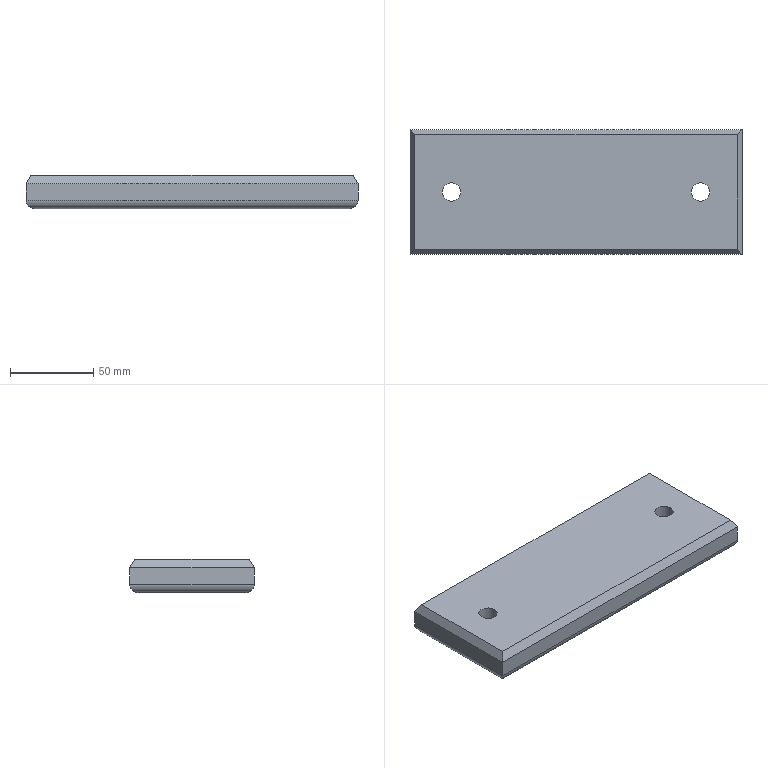Part | NX | features solid 2 | 1 solid | 22 faces | box 200 x 75 x 20 mm | volume 285510 mm3 | plane 12 | cylinder 8 | torus 2 | commonest cylinder face diameters 10 x4 11 x2 17.5 x2
STEP:
#1=CARTESIAN_POINT('',(110.,355.,205.));
#2=VERTEX_POINT('',#1);
#3=CARTESIAN_POINT('',(110.,355.,195.));
#4=VERTEX_POINT('',#3);
#5=CARTESIAN_POINT('',(110.,355.,210.));
#6=DIRECTION('',(0.,0.,-1.));
#7=VECTOR('',#6,1000.);
#8=LINE('',#5,#7);
#9=EDGE_CURVE('',#2,#4,#8,.T.);
#10=ORIENTED_EDGE('',*,*,#9,.F.);
#11=CARTESIAN_POINT('',(310.,355.,205.));
#12=VERTEX_POINT('',#11);
#13=CARTESIAN_POINT('',(230.,355.,205.));
#14=DIRECTION('',(1.,0.,0.));
#15=VECTOR('',#14,1000.);
#16=LINE('',#13,#15);
#17=EDGE_CURVE('',#2,#12,#16,.T.);
#18=ORIENTED_EDGE('',*,*,#17,.T.);
#19=CARTESIAN_POINT('',(310.,355.,195.));
#20=VERTEX_POINT('',#19);
#21=CARTESIAN_POINT('',(310.,355.,210.));
#22=DIRECTION('',(0.,0.,-1.));
#23=VECTOR('',#22,1000.);
#24=LINE('',#21,#23);
#25=EDGE_CURVE('',#12,#20,#24,.T.);
#26=ORIENTED_EDGE('',*,*,#25,.T.);
#27=CARTESIAN_POINT('',(110.,355.,195.));
#28=DIRECTION('',(-1.,0.,0.));
#29=VECTOR('',#28,1000.);
#30=LINE('',#27,#29);
#31=EDGE_CURVE('',#20,#4,#30,.T.);
#32=ORIENTED_EDGE('',*,*,#31,.T.);
#33=EDGE_LOOP('',(#10,#18,#26,#32));
#34=FACE_BOUND('',#33,.T.);
#35=CARTESIAN_POINT('',(230.,355.,210.));
#36=DIRECTION('',(0.,-1.,0.));
#37=DIRECTION('',(0.,0.,-1.));
#38=AXIS2_PLACEMENT_3D('',#35,#36,#37);
#39=PLANE('',#38);
#40=ADVANCED_FACE('',(#34),#39,.F.);
#41=CARTESIAN_POINT('',(110.,280.,205.));
#42=VERTEX_POINT('',#41);
#43=CARTESIAN_POINT('',(110.,280.,195.));
#44=VERTEX_POINT('',#43);
#45=CARTESIAN_POINT('',(110.,280.,210.));
#46=DIRECTION('',(0.,0.,-1.));
#47=VECTOR('',#46,1000.);
#48=LINE('',#45,#47);
#49=EDGE_CURVE('',#42,#44,#48,.T.);
#50=ORIENTED_EDGE('',*,*,#49,.F.);
#51=CARTESIAN_POINT('',(110.,355.,205.));
#52=DIRECTION('',(0.,1.,0.));
#53=VECTOR('',#52,1000.);
#54=LINE('',#51,#53);
#55=EDGE_CURVE('',#42,#2,#54,.T.);
#56=ORIENTED_EDGE('',*,*,#55,.T.);
#57=ORIENTED_EDGE('',*,*,#9,.T.);
#58=CARTESIAN_POINT('',(110.,280.,195.));
#59=DIRECTION('',(0.,-1.,0.));
#60=VECTOR('',#59,1000.);
#61=LINE('',#58,#60);
#62=EDGE_CURVE('',#4,#44,#61,.T.);
#63=ORIENTED_EDGE('',*,*,#62,.T.);
#64=EDGE_LOOP('',(#50,#56,#57,#63));
#65=FACE_BOUND('',#64,.T.);
#66=CARTESIAN_POINT('',(110.,355.,210.));
#67=DIRECTION('',(1.,0.,0.));
#68=DIRECTION('',(0.,0.,1.));
#69=AXIS2_PLACEMENT_3D('',#66,#67,#68);
#70=PLANE('',#69);
#71=ADVANCED_FACE('',(#65),#70,.F.);
#72=CARTESIAN_POINT('',(310.,280.,205.));
#73=VERTEX_POINT('',#72);
#74=CARTESIAN_POINT('',(310.,280.,195.));
#75=VERTEX_POINT('',#74);
#76=CARTESIAN_POINT('',(310.,280.,210.));
#77=DIRECTION('',(0.,0.,-1.));
#78=VECTOR('',#77,1000.);
#79=LINE('',#76,#78);
#80=EDGE_CURVE('',#73,#75,#79,.T.);
#81=ORIENTED_EDGE('',*,*,#80,.F.);
#82=CARTESIAN_POINT('',(110.,280.,205.));
#83=DIRECTION('',(-1.,0.,0.));
#84=VECTOR('',#83,1000.);
#85=LINE('',#82,#84);
#86=EDGE_CURVE('',#73,#42,#85,.T.);
#87=ORIENTED_EDGE('',*,*,#86,.T.);
#88=ORIENTED_EDGE('',*,*,#49,.T.);
#89=CARTESIAN_POINT('',(230.,280.,195.));
#90=DIRECTION('',(-1.,0.,0.));
#91=VECTOR('',#90,1000.);
#92=LINE('',#89,#91);
#93=EDGE_CURVE('',#44,#75,#92,.F.);
#94=ORIENTED_EDGE('',*,*,#93,.T.);
#95=EDGE_LOOP('',(#81,#87,#88,#94));
#96=FACE_BOUND('',#95,.T.);
#97=CARTESIAN_POINT('',(230.,280.,210.));
#98=DIRECTION('',(0.,-1.,0.));
#99=DIRECTION('',(0.,0.,-1.));
#100=AXIS2_PLACEMENT_3D('',#97,#98,#99);
#101=PLANE('',#100);
#102=ADVANCED_FACE('',(#96),#101,.T.);
#103=ORIENTED_EDGE('',*,*,#25,.F.);
#104=CARTESIAN_POINT('',(310.,280.,205.));
#105=DIRECTION('',(0.,-1.,0.));
#106=VECTOR('',#105,1000.);
#107=LINE('',#104,#106);
#108=EDGE_CURVE('',#12,#73,#107,.T.);
#109=ORIENTED_EDGE('',*,*,#108,.T.);
#110=ORIENTED_EDGE('',*,*,#80,.T.);
#111=CARTESIAN_POINT('',(310.,355.,195.));
#112=DIRECTION('',(0.,-1.,0.));
#113=VECTOR('',#112,1000.);
#114=LINE('',#111,#113);
#115=EDGE_CURVE('',#75,#20,#114,.F.);
#116=ORIENTED_EDGE('',*,*,#115,.T.);
#117=EDGE_LOOP('',(#103,#109,#110,#116));
#118=FACE_BOUND('',#117,.T.);
#119=CARTESIAN_POINT('',(310.,355.,210.));
#120=DIRECTION('',(1.,0.,0.));
#121=DIRECTION('',(0.,0.,1.));
#122=AXIS2_PLACEMENT_3D('',#119,#120,#121);
#123=PLANE('',#122);
#124=ADVANCED_FACE('',(#118),#123,.T.);
#125=CARTESIAN_POINT('',(113.,283.,210.));
#126=VERTEX_POINT('',#125);
#127=CARTESIAN_POINT('',(307.,283.,210.));
#128=VERTEX_POINT('',#127);
#129=CARTESIAN_POINT('',(310.,283.,210.));
#130=DIRECTION('',(1.,0.,0.));
#131=VECTOR('',#130,1000.);
#132=LINE('',#129,#131);
#133=EDGE_CURVE('',#126,#128,#132,.T.);
#134=ORIENTED_EDGE('',*,*,#133,.T.);
#135=CARTESIAN_POINT('',(307.,352.,210.));
#136=VERTEX_POINT('',#135);
#137=CARTESIAN_POINT('',(307.,355.,210.));
#138=DIRECTION('',(0.,1.,0.));
#139=VECTOR('',#138,1000.);
#140=LINE('',#137,#139);
#141=EDGE_CURVE('',#128,#136,#140,.T.);
#142=ORIENTED_EDGE('',*,*,#141,.T.);
#143=CARTESIAN_POINT('',(113.,352.,210.));
#144=VERTEX_POINT('',#143);
#145=CARTESIAN_POINT('',(230.,352.,210.));
#146=DIRECTION('',(-1.,0.,0.));
#147=VECTOR('',#146,1000.);
#148=LINE('',#145,#147);
#149=EDGE_CURVE('',#136,#144,#148,.T.);
#150=ORIENTED_EDGE('',*,*,#149,.T.);
#151=CARTESIAN_POINT('',(113.,355.,210.));
#152=DIRECTION('',(0.,-1.,0.));
#153=VECTOR('',#152,1000.);
#154=LINE('',#151,#153);
#155=EDGE_CURVE('',#144,#126,#154,.T.);
#156=ORIENTED_EDGE('',*,*,#155,.T.);
#157=EDGE_LOOP('',(#134,#142,#150,#156));
#158=FACE_BOUND('',#157,.T.);
#159=CARTESIAN_POINT('',(290.5,317.5,210.));
#160=VERTEX_POINT('',#159);
#161=CARTESIAN_POINT('',(285.,317.5,210.));
#162=DIRECTION('',(0.,0.,-1.));
#163=DIRECTION('',(1.,0.,0.));
#164=AXIS2_PLACEMENT_3D('',#161,#162,#163);
#165=CIRCLE('',#164,5.5);
#166=EDGE_CURVE('',#160,#160,#165,.T.);
#167=ORIENTED_EDGE('',*,*,#166,.T.);
#168=EDGE_LOOP('',(#167));
#169=FACE_BOUND('',#168,.T.);
#170=CARTESIAN_POINT('',(140.5,317.5,210.));
#171=VERTEX_POINT('',#170);
#172=CARTESIAN_POINT('',(135.,317.5,210.));
#173=DIRECTION('',(0.,0.,-1.));
#174=DIRECTION('',(1.,0.,0.));
#175=AXIS2_PLACEMENT_3D('',#172,#173,#174);
#176=CIRCLE('',#175,5.5);
#177=EDGE_CURVE('',#171,#171,#176,.T.);
#178=ORIENTED_EDGE('',*,*,#177,.T.);
#179=EDGE_LOOP('',(#178));
#180=FACE_BOUND('',#179,.T.);
#181=CARTESIAN_POINT('',(230.,355.,210.));
#182=DIRECTION('',(0.,0.,-1.));
#183=DIRECTION('',(-1.,0.,0.));
#184=AXIS2_PLACEMENT_3D('',#181,#182,#183);
#185=PLANE('',#184);
#186=ADVANCED_FACE('',(#158,#169,#180),#185,.F.);
#187=CARTESIAN_POINT('',(296.75,317.5,190.));
#188=VERTEX_POINT('',#187);
#189=CARTESIAN_POINT('',(285.,317.5,190.));
#190=DIRECTION('',(0.,0.,-1.));
#191=DIRECTION('',(1.,0.,0.));
#192=AXIS2_PLACEMENT_3D('',#189,#190,#191);
#193=CIRCLE('',#192,11.75);
#194=EDGE_CURVE('',#188,#188,#193,.F.);
#195=ORIENTED_EDGE('',*,*,#194,.T.);
#196=EDGE_LOOP('',(#195));
#197=FACE_BOUND('',#196,.T.);
#198=CARTESIAN_POINT('',(146.75,317.5,190.));
#199=VERTEX_POINT('',#198);
#200=CARTESIAN_POINT('',(135.,317.5,190.));
#201=DIRECTION('',(0.,0.,-1.));
#202=DIRECTION('',(1.,0.,0.));
#203=AXIS2_PLACEMENT_3D('',#200,#201,#202);
#204=CIRCLE('',#203,11.75);
#205=EDGE_CURVE('',#199,#199,#204,.F.);
#206=ORIENTED_EDGE('',*,*,#205,.T.);
#207=EDGE_LOOP('',(#206));
#208=FACE_BOUND('',#207,.T.);
#209=CARTESIAN_POINT('',(115.,350.,190.));
#210=VERTEX_POINT('',#209);
#211=CARTESIAN_POINT('',(305.,350.,190.));
#212=VERTEX_POINT('',#211);
#213=CARTESIAN_POINT('',(310.,350.,190.));
#214=DIRECTION('',(-1.,0.,0.));
#215=VECTOR('',#214,1000.);
#216=LINE('',#213,#215);
#217=EDGE_CURVE('',#210,#212,#216,.F.);
#218=ORIENTED_EDGE('',*,*,#217,.T.);
#219=CARTESIAN_POINT('',(305.,285.,190.));
#220=VERTEX_POINT('',#219);
#221=CARTESIAN_POINT('',(305.,355.,190.));
#222=DIRECTION('',(0.,-1.,0.));
#223=VECTOR('',#222,1000.);
#224=LINE('',#221,#223);
#225=EDGE_CURVE('',#212,#220,#224,.T.);
#226=ORIENTED_EDGE('',*,*,#225,.T.);
#227=CARTESIAN_POINT('',(115.,285.,190.));
#228=VERTEX_POINT('',#227);
#229=CARTESIAN_POINT('',(230.,285.,190.));
#230=DIRECTION('',(-1.,0.,0.));
#231=VECTOR('',#230,1000.);
#232=LINE('',#229,#231);
#233=EDGE_CURVE('',#220,#228,#232,.T.);
#234=ORIENTED_EDGE('',*,*,#233,.T.);
#235=CARTESIAN_POINT('',(115.,355.,190.));
#236=DIRECTION('',(0.,-1.,0.));
#237=VECTOR('',#236,1000.);
#238=LINE('',#235,#237);
#239=EDGE_CURVE('',#228,#210,#238,.F.);
#240=ORIENTED_EDGE('',*,*,#239,.T.);
#241=EDGE_LOOP('',(#218,#226,#234,#240));
#242=FACE_BOUND('',#241,.T.);
#243=CARTESIAN_POINT('',(230.,355.,190.));
#244=DIRECTION('',(0.,0.,-1.));
#245=DIRECTION('',(-1.,0.,0.));
#246=AXIS2_PLACEMENT_3D('',#243,#244,#245);
#247=PLANE('',#246);
#248=ADVANCED_FACE('',(#197,#208,#242),#247,.T.);
#249=CARTESIAN_POINT('',(129.5,317.5,202.));
#250=VERTEX_POINT('',#249);
#251=CARTESIAN_POINT('',(135.,317.5,202.));
#252=DIRECTION('',(0.,0.,1.));
#253=DIRECTION('',(-1.,0.,0.));
#254=AXIS2_PLACEMENT_3D('',#251,#252,#253);
#255=CIRCLE('',#254,5.5);
#256=EDGE_CURVE('',#250,#250,#255,.T.);
#257=ORIENTED_EDGE('',*,*,#256,.F.);
#258=EDGE_LOOP('',(#257));
#259=FACE_BOUND('',#258,.T.);
#260=ORIENTED_EDGE('',*,*,#177,.F.);
#261=EDGE_LOOP('',(#260));
#262=FACE_BOUND('',#261,.T.);
#263=CARTESIAN_POINT('',(135.,317.5,240.));
#264=DIRECTION('',(0.,0.,1.));
#265=DIRECTION('',(-1.,0.,0.));
#266=AXIS2_PLACEMENT_3D('',#263,#264,#265);
#267=CYLINDRICAL_SURFACE('',#266,5.5);
#268=ADVANCED_FACE('',(#259,#262),#267,.F.);
#269=ORIENTED_EDGE('',*,*,#256,.T.);
#270=EDGE_LOOP('',(#269));
#271=FACE_BOUND('',#270,.T.);
#272=CARTESIAN_POINT('',(126.25,317.5,202.));
#273=VERTEX_POINT('',#272);
#274=CARTESIAN_POINT('',(135.,317.5,202.));
#275=DIRECTION('',(0.,0.,1.));
#276=DIRECTION('',(-1.,0.,0.));
#277=AXIS2_PLACEMENT_3D('',#274,#275,#276);
#278=CIRCLE('',#277,8.75);
#279=EDGE_CURVE('',#273,#273,#278,.T.);
#280=ORIENTED_EDGE('',*,*,#279,.F.);
#281=EDGE_LOOP('',(#280));
#282=FACE_BOUND('',#281,.T.);
#283=CARTESIAN_POINT('',(135.,317.5,202.));
#284=DIRECTION('',(0.,0.,1.));
#285=DIRECTION('',(-1.,0.,0.));
#286=AXIS2_PLACEMENT_3D('',#283,#284,#285);
#287=PLANE('',#286);
#288=ADVANCED_FACE('',(#271,#282),#287,.F.);
#289=CARTESIAN_POINT('',(143.75,317.5,193.));
#290=VERTEX_POINT('',#289);
#291=CARTESIAN_POINT('',(135.,317.5,193.));
#292=DIRECTION('',(0.,0.,-1.));
#293=DIRECTION('',(1.,0.,0.));
#294=AXIS2_PLACEMENT_3D('',#291,#292,#293);
#295=CIRCLE('',#294,8.75);
#296=EDGE_CURVE('',#290,#290,#295,.T.);
#297=ORIENTED_EDGE('',*,*,#296,.T.);
#298=EDGE_LOOP('',(#297));
#299=FACE_BOUND('',#298,.T.);
#300=ORIENTED_EDGE('',*,*,#279,.T.);
#301=EDGE_LOOP('',(#300));
#302=FACE_BOUND('',#301,.T.);
#303=CARTESIAN_POINT('',(135.,317.5,190.));
#304=DIRECTION('',(0.,0.,1.));
#305=DIRECTION('',(-1.,0.,0.));
#306=AXIS2_PLACEMENT_3D('',#303,#304,#305);
#307=CYLINDRICAL_SURFACE('',#306,8.75);
#308=ADVANCED_FACE('',(#299,#302),#307,.F.);
#309=CARTESIAN_POINT('',(279.5,317.5,202.));
#310=VERTEX_POINT('',#309);
#311=CARTESIAN_POINT('',(285.,317.5,202.));
#312=DIRECTION('',(0.,0.,1.));
#313=DIRECTION('',(-1.,0.,0.));
#314=AXIS2_PLACEMENT_3D('',#311,#312,#313);
#315=CIRCLE('',#314,5.5);
#316=EDGE_CURVE('',#310,#310,#315,.T.);
#317=ORIENTED_EDGE('',*,*,#316,.F.);
#318=EDGE_LOOP('',(#317));
#319=FACE_BOUND('',#318,.T.);
#320=ORIENTED_EDGE('',*,*,#166,.F.);
#321=EDGE_LOOP('',(#320));
#322=FACE_BOUND('',#321,.T.);
#323=CARTESIAN_POINT('',(285.,317.5,240.));
#324=DIRECTION('',(0.,0.,1.));
#325=DIRECTION('',(-1.,0.,0.));
#326=AXIS2_PLACEMENT_3D('',#323,#324,#325);
#327=CYLINDRICAL_SURFACE('',#326,5.5);
#328=ADVANCED_FACE('',(#319,#322),#327,.F.);
#329=ORIENTED_EDGE('',*,*,#316,.T.);
#330=EDGE_LOOP('',(#329));
#331=FACE_BOUND('',#330,.T.);
#332=CARTESIAN_POINT('',(276.25,317.5,202.));
#333=VERTEX_POINT('',#332);
#334=CARTESIAN_POINT('',(285.,317.5,202.));
#335=DIRECTION('',(0.,0.,1.));
#336=DIRECTION('',(-1.,0.,0.));
#337=AXIS2_PLACEMENT_3D('',#334,#335,#336);
#338=CIRCLE('',#337,8.75);
#339=EDGE_CURVE('',#333,#333,#338,.T.);
#340=ORIENTED_EDGE('',*,*,#339,.F.);
#341=EDGE_LOOP('',(#340));
#342=FACE_BOUND('',#341,.T.);
#343=CARTESIAN_POINT('',(285.,317.5,202.));
#344=DIRECTION('',(0.,0.,1.));
#345=DIRECTION('',(-1.,0.,0.));
#346=AXIS2_PLACEMENT_3D('',#343,#344,#345);
#347=PLANE('',#346);
#348=ADVANCED_FACE('',(#331,#342),#347,.F.);
#349=CARTESIAN_POINT('',(293.75,317.5,193.));
#350=VERTEX_POINT('',#349);
#351=CARTESIAN_POINT('',(285.,317.5,193.));
#352=DIRECTION('',(0.,0.,-1.));
#353=DIRECTION('',(1.,0.,0.));
#354=AXIS2_PLACEMENT_3D('',#351,#352,#353);
#355=CIRCLE('',#354,8.75);
#356=EDGE_CURVE('',#350,#350,#355,.T.);
#357=ORIENTED_EDGE('',*,*,#356,.T.);
#358=EDGE_LOOP('',(#357));
#359=FACE_BOUND('',#358,.T.);
#360=ORIENTED_EDGE('',*,*,#339,.T.);
#361=EDGE_LOOP('',(#360));
#362=FACE_BOUND('',#361,.T.);
#363=CARTESIAN_POINT('',(285.,317.5,190.));
#364=DIRECTION('',(0.,0.,1.));
#365=DIRECTION('',(-1.,0.,0.));
#366=AXIS2_PLACEMENT_3D('',#363,#364,#365);
#367=CYLINDRICAL_SURFACE('',#366,8.75);
#368=ADVANCED_FACE('',(#359,#362),#367,.F.);
#369=CARTESIAN_POINT('',(115.,285.,195.));
#370=DIRECTION('',(-0.7071,0.7071,0.));
#371=DIRECTION('',(0.7071,0.7071,0.));
#372=AXIS2_PLACEMENT_3D('',#369,#370,#371);
#373=ELLIPSE('',#372,7.071,5.);
#374=EDGE_CURVE('',#44,#228,#373,.F.);
#375=ORIENTED_EDGE('',*,*,#374,.F.);
#376=ORIENTED_EDGE('',*,*,#62,.F.);
#377=CARTESIAN_POINT('',(115.,350.,195.));
#378=DIRECTION('',(0.7071,0.7071,0.));
#379=DIRECTION('',(0.7071,-0.7071,0.));
#380=AXIS2_PLACEMENT_3D('',#377,#378,#379);
#381=ELLIPSE('',#380,7.071,5.);
#382=EDGE_CURVE('',#210,#4,#381,.T.);
#383=ORIENTED_EDGE('',*,*,#382,.F.);
#384=ORIENTED_EDGE('',*,*,#239,.F.);
#385=EDGE_LOOP('',(#375,#376,#383,#384));
#386=FACE_BOUND('',#385,.T.);
#387=CARTESIAN_POINT('',(115.,355.,195.));
#388=DIRECTION('',(0.,1.,0.));
#389=DIRECTION('',(0.,0.,1.));
#390=AXIS2_PLACEMENT_3D('',#387,#388,#389);
#391=CYLINDRICAL_SURFACE('',#390,5.);
#392=ADVANCED_FACE('',(#386),#391,.T.);
#393=ORIENTED_EDGE('',*,*,#382,.T.);
#394=ORIENTED_EDGE('',*,*,#31,.F.);
#395=CARTESIAN_POINT('',(305.,350.,195.));
#396=DIRECTION('',(0.7071,-0.7071,0.));
#397=DIRECTION('',(0.7071,0.7071,0.));
#398=AXIS2_PLACEMENT_3D('',#395,#396,#397);
#399=ELLIPSE('',#398,7.071,5.);
#400=EDGE_CURVE('',#212,#20,#399,.T.);
#401=ORIENTED_EDGE('',*,*,#400,.F.);
#402=ORIENTED_EDGE('',*,*,#217,.F.);
#403=EDGE_LOOP('',(#393,#394,#401,#402));
#404=FACE_BOUND('',#403,.T.);
#405=CARTESIAN_POINT('',(230.,350.,195.));
#406=DIRECTION('',(1.,0.,0.));
#407=DIRECTION('',(0.,0.,1.));
#408=AXIS2_PLACEMENT_3D('',#405,#406,#407);
#409=CYLINDRICAL_SURFACE('',#408,5.);
#410=ADVANCED_FACE('',(#404),#409,.T.);
#411=ORIENTED_EDGE('',*,*,#374,.T.);
#412=ORIENTED_EDGE('',*,*,#233,.F.);
#413=CARTESIAN_POINT('',(305.,285.,195.));
#414=DIRECTION('',(-0.7071,-0.7071,0.));
#415=DIRECTION('',(-0.7071,0.7071,0.));
#416=AXIS2_PLACEMENT_3D('',#413,#414,#415);
#417=ELLIPSE('',#416,7.071,5.);
#418=EDGE_CURVE('',#75,#220,#417,.F.);
#419=ORIENTED_EDGE('',*,*,#418,.F.);
#420=ORIENTED_EDGE('',*,*,#93,.F.);
#421=EDGE_LOOP('',(#411,#412,#419,#420));
#422=FACE_BOUND('',#421,.T.);
#423=CARTESIAN_POINT('',(230.,285.,195.));
#424=DIRECTION('',(-1.,0.,0.));
#425=DIRECTION('',(0.,0.,-1.));
#426=AXIS2_PLACEMENT_3D('',#423,#424,#425);
#427=CYLINDRICAL_SURFACE('',#426,5.);
#428=ADVANCED_FACE('',(#422),#427,.T.);
#429=ORIENTED_EDGE('',*,*,#400,.T.);
#430=ORIENTED_EDGE('',*,*,#115,.F.);
#431=ORIENTED_EDGE('',*,*,#418,.T.);
#432=ORIENTED_EDGE('',*,*,#225,.F.);
#433=EDGE_LOOP('',(#429,#430,#431,#432));
#434=FACE_BOUND('',#433,.T.);
#435=CARTESIAN_POINT('',(305.,355.,195.));
#436=DIRECTION('',(0.,-1.,0.));
#437=DIRECTION('',(0.,0.,-1.));
#438=AXIS2_PLACEMENT_3D('',#435,#436,#437);
#439=CYLINDRICAL_SURFACE('',#438,5.);
#440=ADVANCED_FACE('',(#434),#439,.T.);
#441=ORIENTED_EDGE('',*,*,#356,.F.);
#442=EDGE_LOOP('',(#441));
#443=FACE_BOUND('',#442,.T.);
#444=ORIENTED_EDGE('',*,*,#194,.F.);
#445=EDGE_LOOP('',(#444));
#446=FACE_BOUND('',#445,.T.);
#447=CARTESIAN_POINT('',(285.,317.5,193.));
#448=DIRECTION('',(0.,0.,-1.));
#449=DIRECTION('',(1.,0.,0.));
#450=AXIS2_PLACEMENT_3D('',#447,#448,#449);
#451=TOROIDAL_SURFACE('',#450,11.75,3.);
#452=ADVANCED_FACE('',(#443,#446),#451,.T.);
#453=ORIENTED_EDGE('',*,*,#296,.F.);
#454=EDGE_LOOP('',(#453));
#455=FACE_BOUND('',#454,.T.);
#456=ORIENTED_EDGE('',*,*,#205,.F.);
#457=EDGE_LOOP('',(#456));
#458=FACE_BOUND('',#457,.T.);
#459=CARTESIAN_POINT('',(135.,317.5,193.));
#460=DIRECTION('',(0.,0.,-1.));
#461=DIRECTION('',(1.,0.,0.));
#462=AXIS2_PLACEMENT_3D('',#459,#460,#461);
#463=TOROIDAL_SURFACE('',#462,11.75,3.);
#464=ADVANCED_FACE('',(#455,#458),#463,.T.);
#465=CARTESIAN_POINT('',(128.07,298.07,235.116));
#466=DIRECTION('',(-0.4575,-0.4575,-0.7625));
#467=VECTOR('',#466,1000.);
#468=LINE('',#465,#467);
#469=EDGE_CURVE('',#126,#42,#468,.T.);
#470=ORIENTED_EDGE('',*,*,#469,.F.);
#471=ORIENTED_EDGE('',*,*,#155,.F.);
#472=CARTESIAN_POINT('',(137.488,327.512,250.814));
#473=DIRECTION('',(0.4575,-0.4575,0.7625));
#474=VECTOR('',#473,1000.);
#475=LINE('',#472,#474);
#476=EDGE_CURVE('',#2,#144,#475,.T.);
#477=ORIENTED_EDGE('',*,*,#476,.F.);
#478=ORIENTED_EDGE('',*,*,#55,.F.);
#479=EDGE_LOOP('',(#470,#471,#477,#478));
#480=FACE_BOUND('',#479,.T.);
#481=CARTESIAN_POINT('',(113.,355.,210.));
#482=DIRECTION('',(0.8575,0.,-0.5145));
#483=DIRECTION('',(0.5145,0.,0.8575));
#484=AXIS2_PLACEMENT_3D('',#481,#482,#483);
#485=PLANE('',#484);
#486=ADVANCED_FACE('',(#480),#485,.F.);
#487=ORIENTED_EDGE('',*,*,#476,.T.);
#488=ORIENTED_EDGE('',*,*,#149,.F.);
#489=CARTESIAN_POINT('',(290.884,335.884,236.86));
#490=DIRECTION('',(-0.4575,-0.4575,0.7625));
#491=VECTOR('',#490,1000.);
#492=LINE('',#489,#491);
#493=EDGE_CURVE('',#12,#136,#492,.T.);
#494=ORIENTED_EDGE('',*,*,#493,.F.);
#495=ORIENTED_EDGE('',*,*,#17,.F.);
#496=EDGE_LOOP('',(#487,#488,#494,#495));
#497=FACE_BOUND('',#496,.T.);
#498=CARTESIAN_POINT('',(230.,352.,210.));
#499=DIRECTION('',(0.,-0.8575,-0.5145));
#500=DIRECTION('',(0.,0.5145,-0.8575));
#501=AXIS2_PLACEMENT_3D('',#498,#499,#500);
#502=PLANE('',#501);
#503=ADVANCED_FACE('',(#497),#502,.F.);
#504=ORIENTED_EDGE('',*,*,#469,.T.);
#505=ORIENTED_EDGE('',*,*,#86,.F.);
#506=CARTESIAN_POINT('',(293.256,296.744,232.907));
#507=DIRECTION('',(-0.4575,0.4575,0.7625));
#508=VECTOR('',#507,1000.);
#509=LINE('',#506,#508);
#510=EDGE_CURVE('',#128,#73,#509,.F.);
#511=ORIENTED_EDGE('',*,*,#510,.F.);
#512=ORIENTED_EDGE('',*,*,#133,.F.);
#513=EDGE_LOOP('',(#504,#505,#511,#512));
#514=FACE_BOUND('',#513,.T.);
#515=CARTESIAN_POINT('',(230.,280.,205.));
#516=DIRECTION('',(0.,-0.8575,0.5145));
#517=DIRECTION('',(0.,-0.5145,-0.8575));
#518=AXIS2_PLACEMENT_3D('',#515,#516,#517);
#519=PLANE('',#518);
#520=ADVANCED_FACE('',(#514),#519,.T.);
#521=ORIENTED_EDGE('',*,*,#493,.T.);
#522=ORIENTED_EDGE('',*,*,#141,.F.);
#523=ORIENTED_EDGE('',*,*,#510,.T.);
#524=ORIENTED_EDGE('',*,*,#108,.F.);
#525=EDGE_LOOP('',(#521,#522,#523,#524));
#526=FACE_BOUND('',#525,.T.);
#527=CARTESIAN_POINT('',(310.,355.,205.));
#528=DIRECTION('',(0.8575,0.,0.5145));
#529=DIRECTION('',(-0.5145,0.,0.8575));
#530=AXIS2_PLACEMENT_3D('',#527,#528,#529);
#531=PLANE('',#530);
#532=ADVANCED_FACE('',(#526),#531,.T.);
#533=CLOSED_SHELL('',(#40,#71,#102,#124,#186,#248,#268,#288,#308,#328,#348,#368,#392,#410,#428,#440,#452,#464,#486,#503,#520,#532));
#534=MANIFOLD_SOLID_BREP('',#533);
#535=(LENGTH_UNIT()NAMED_UNIT(*)SI_UNIT(.MILLI.,.METRE.));
#536=UNCERTAINTY_MEASURE_WITH_UNIT(LENGTH_MEASURE(0.00001),#535,'','');
#537=(NAMED_UNIT(*)PLANE_ANGLE_UNIT()SI_UNIT($,.RADIAN.));
#538=(NAMED_UNIT(*)SI_UNIT($,.STERADIAN.)SOLID_ANGLE_UNIT());
#539=(GEOMETRIC_REPRESENTATION_CONTEXT(3)GLOBAL_UNCERTAINTY_ASSIGNED_CONTEXT((#536))GLOBAL_UNIT_ASSIGNED_CONTEXT((#535,#537,#538))REPRESENTATION_CONTEXT('',''));
#540=ADVANCED_BREP_SHAPE_REPRESENTATION('',(#534),#539);